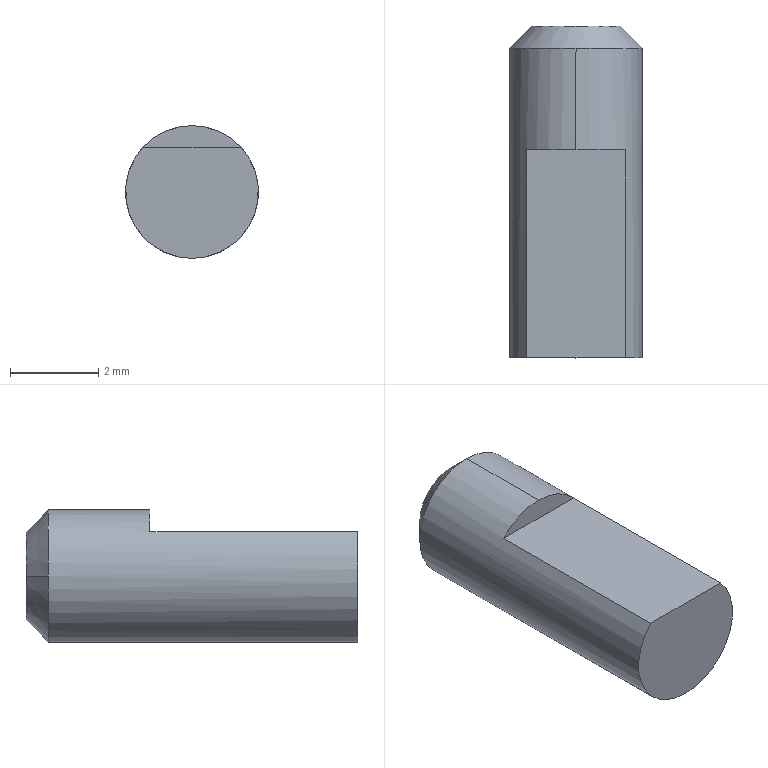Part | NX | 1 solid | 8 faces | box 3 x 7.5 x 3 mm | volume 48.328 mm3 | plane 4 | cylinder 2 | cone 2 | commonest cylinder face diameters 3 x2
STEP:
#1=CARTESIAN_POINT('',(0.171,-56.129,15.403));
#2=VERTEX_POINT('',#1);
#3=CARTESIAN_POINT('',(-1.329,-56.129,16.903));
#4=VERTEX_POINT('',#3);
#5=CARTESIAN_POINT('',(-1.329,-56.129,15.403));
#6=DIRECTION('',(0.,-1.,0.));
#7=DIRECTION('',(1.,0.,0.));
#8=AXIS2_PLACEMENT_3D('',#5,#6,#7);
#9=CIRCLE('',#8,1.5);
#10=EDGE_CURVE('',#2,#4,#9,.T.);
#11=ORIENTED_EDGE('',*,*,#10,.T.);
#12=CARTESIAN_POINT('',(-1.329,-58.429,16.903));
#13=VERTEX_POINT('',#12);
#14=CARTESIAN_POINT('',(-1.329,-63.129,16.903));
#15=DIRECTION('',(0.,-1.,0.));
#16=VECTOR('',#15,1000.);
#17=LINE('',#14,#16);
#18=EDGE_CURVE('',#4,#13,#17,.T.);
#19=ORIENTED_EDGE('',*,*,#18,.T.);
#20=CARTESIAN_POINT('',(-0.211,-58.429,16.403));
#21=VERTEX_POINT('',#20);
#22=CARTESIAN_POINT('',(-1.329,-58.429,15.403));
#23=DIRECTION('',(0.,-1.,0.));
#24=DIRECTION('',(0.,0.,1.));
#25=AXIS2_PLACEMENT_3D('',#22,#23,#24);
#26=CIRCLE('',#25,1.5);
#27=EDGE_CURVE('',#21,#13,#26,.T.);
#28=ORIENTED_EDGE('',*,*,#27,.F.);
#29=CARTESIAN_POINT('',(-0.211,-63.129,16.403));
#30=VERTEX_POINT('',#29);
#31=CARTESIAN_POINT('',(-0.211,-63.129,16.403));
#32=DIRECTION('',(0.,-1.,0.));
#33=VECTOR('',#32,1000.);
#34=LINE('',#31,#33);
#35=EDGE_CURVE('',#21,#30,#34,.T.);
#36=ORIENTED_EDGE('',*,*,#35,.T.);
#37=CARTESIAN_POINT('',(-1.329,-63.129,13.903));
#38=VERTEX_POINT('',#37);
#39=CARTESIAN_POINT('',(-1.329,-63.129,15.403));
#40=DIRECTION('',(0.,-1.,0.));
#41=DIRECTION('',(0.,0.,1.));
#42=AXIS2_PLACEMENT_3D('',#39,#40,#41);
#43=CIRCLE('',#42,1.5);
#44=EDGE_CURVE('',#38,#30,#43,.T.);
#45=ORIENTED_EDGE('',*,*,#44,.F.);
#46=CARTESIAN_POINT('',(-1.329,-56.129,13.903));
#47=VERTEX_POINT('',#46);
#48=CARTESIAN_POINT('',(-1.329,-63.129,13.903));
#49=DIRECTION('',(0.,-1.,0.));
#50=VECTOR('',#49,1000.);
#51=LINE('',#48,#50);
#52=EDGE_CURVE('',#47,#38,#51,.T.);
#53=ORIENTED_EDGE('',*,*,#52,.F.);
#54=CARTESIAN_POINT('',(-1.329,-56.129,15.403));
#55=DIRECTION('',(0.,-1.,0.));
#56=DIRECTION('',(1.,0.,0.));
#57=AXIS2_PLACEMENT_3D('',#54,#55,#56);
#58=CIRCLE('',#57,1.5);
#59=EDGE_CURVE('',#47,#2,#58,.T.);
#60=ORIENTED_EDGE('',*,*,#59,.T.);
#61=EDGE_LOOP('',(#11,#19,#28,#36,#45,#53,#60));
#62=FACE_BOUND('',#61,.T.);
#63=CARTESIAN_POINT('',(-1.329,-63.129,15.403));
#64=DIRECTION('',(0.,-1.,0.));
#65=DIRECTION('',(0.,0.,1.));
#66=AXIS2_PLACEMENT_3D('',#63,#64,#65);
#67=CYLINDRICAL_SURFACE('',#66,1.5);
#68=ADVANCED_FACE('',(#62),#67,.T.);
#69=CARTESIAN_POINT('',(-2.447,-58.429,16.403));
#70=VERTEX_POINT('',#69);
#71=CARTESIAN_POINT('',(-1.329,-58.429,15.403));
#72=DIRECTION('',(0.,-1.,0.));
#73=DIRECTION('',(0.,0.,1.));
#74=AXIS2_PLACEMENT_3D('',#71,#72,#73);
#75=CIRCLE('',#74,1.5);
#76=EDGE_CURVE('',#13,#70,#75,.T.);
#77=ORIENTED_EDGE('',*,*,#76,.F.);
#78=ORIENTED_EDGE('',*,*,#18,.F.);
#79=CARTESIAN_POINT('',(-2.829,-56.129,15.403));
#80=VERTEX_POINT('',#79);
#81=CARTESIAN_POINT('',(-1.329,-56.129,15.403));
#82=DIRECTION('',(0.,-1.,0.));
#83=DIRECTION('',(1.,0.,0.));
#84=AXIS2_PLACEMENT_3D('',#81,#82,#83);
#85=CIRCLE('',#84,1.5);
#86=EDGE_CURVE('',#4,#80,#85,.T.);
#87=ORIENTED_EDGE('',*,*,#86,.T.);
#88=CARTESIAN_POINT('',(-1.329,-56.129,15.403));
#89=DIRECTION('',(0.,-1.,0.));
#90=DIRECTION('',(1.,0.,0.));
#91=AXIS2_PLACEMENT_3D('',#88,#89,#90);
#92=CIRCLE('',#91,1.5);
#93=EDGE_CURVE('',#80,#47,#92,.T.);
#94=ORIENTED_EDGE('',*,*,#93,.T.);
#95=ORIENTED_EDGE('',*,*,#52,.T.);
#96=CARTESIAN_POINT('',(-2.447,-63.129,16.403));
#97=VERTEX_POINT('',#96);
#98=CARTESIAN_POINT('',(-1.329,-63.129,15.403));
#99=DIRECTION('',(0.,-1.,0.));
#100=DIRECTION('',(0.,0.,1.));
#101=AXIS2_PLACEMENT_3D('',#98,#99,#100);
#102=CIRCLE('',#101,1.5);
#103=EDGE_CURVE('',#97,#38,#102,.T.);
#104=ORIENTED_EDGE('',*,*,#103,.F.);
#105=CARTESIAN_POINT('',(-2.447,-63.129,16.403));
#106=DIRECTION('',(0.,-1.,0.));
#107=VECTOR('',#106,1000.);
#108=LINE('',#105,#107);
#109=EDGE_CURVE('',#70,#97,#108,.T.);
#110=ORIENTED_EDGE('',*,*,#109,.F.);
#111=EDGE_LOOP('',(#77,#78,#87,#94,#95,#104,#110));
#112=FACE_BOUND('',#111,.T.);
#113=CARTESIAN_POINT('',(-1.329,-63.129,15.403));
#114=DIRECTION('',(0.,-1.,0.));
#115=DIRECTION('',(0.,0.,1.));
#116=AXIS2_PLACEMENT_3D('',#113,#114,#115);
#117=CYLINDRICAL_SURFACE('',#116,1.5);
#118=ADVANCED_FACE('',(#112),#117,.T.);
#119=CARTESIAN_POINT('',(-0.329,-55.629,15.403));
#120=VERTEX_POINT('',#119);
#121=CARTESIAN_POINT('',(-2.329,-55.629,15.403));
#122=VERTEX_POINT('',#121);
#123=CARTESIAN_POINT('',(-1.329,-55.629,15.403));
#124=DIRECTION('',(0.,-1.,0.));
#125=DIRECTION('',(1.,0.,0.));
#126=AXIS2_PLACEMENT_3D('',#123,#124,#125);
#127=CIRCLE('',#126,1.);
#128=EDGE_CURVE('',#120,#122,#127,.T.);
#129=ORIENTED_EDGE('',*,*,#128,.F.);
#130=CARTESIAN_POINT('',(-1.329,-55.629,15.403));
#131=DIRECTION('',(0.,-1.,0.));
#132=DIRECTION('',(1.,0.,0.));
#133=AXIS2_PLACEMENT_3D('',#130,#131,#132);
#134=CIRCLE('',#133,1.);
#135=EDGE_CURVE('',#122,#120,#134,.T.);
#136=ORIENTED_EDGE('',*,*,#135,.F.);
#137=EDGE_LOOP('',(#129,#136));
#138=FACE_BOUND('',#137,.T.);
#139=CARTESIAN_POINT('',(4.423,-55.629,12.937));
#140=DIRECTION('',(0.,-1.,0.));
#141=DIRECTION('',(-1.,0.,0.));
#142=AXIS2_PLACEMENT_3D('',#139,#140,#141);
#143=PLANE('',#142);
#144=ADVANCED_FACE('',(#138),#143,.F.);
#145=ORIENTED_EDGE('',*,*,#128,.T.);
#146=CARTESIAN_POINT('',(-2.329,-55.629,15.403));
#147=DIRECTION('',(-0.7071,-0.7071,0.));
#148=VECTOR('',#147,1000.);
#149=LINE('',#146,#148);
#150=EDGE_CURVE('',#122,#80,#149,.T.);
#151=ORIENTED_EDGE('',*,*,#150,.T.);
#152=ORIENTED_EDGE('',*,*,#86,.F.);
#153=ORIENTED_EDGE('',*,*,#10,.F.);
#154=CARTESIAN_POINT('',(-0.329,-55.629,15.403));
#155=DIRECTION('',(0.7071,-0.7071,0.));
#156=VECTOR('',#155,1000.);
#157=LINE('',#154,#156);
#158=EDGE_CURVE('',#120,#2,#157,.T.);
#159=ORIENTED_EDGE('',*,*,#158,.F.);
#160=EDGE_LOOP('',(#145,#151,#152,#153,#159));
#161=FACE_BOUND('',#160,.T.);
#162=CARTESIAN_POINT('',(-1.329,-55.629,15.403));
#163=DIRECTION('',(0.,-1.,0.));
#164=DIRECTION('',(1.,0.,0.));
#165=AXIS2_PLACEMENT_3D('',#162,#163,#164);
#166=CONICAL_SURFACE('',#165,1.,0.7854);
#167=ADVANCED_FACE('',(#161),#166,.T.);
#168=ORIENTED_EDGE('',*,*,#158,.T.);
#169=ORIENTED_EDGE('',*,*,#59,.F.);
#170=ORIENTED_EDGE('',*,*,#93,.F.);
#171=ORIENTED_EDGE('',*,*,#150,.F.);
#172=ORIENTED_EDGE('',*,*,#135,.T.);
#173=EDGE_LOOP('',(#168,#169,#170,#171,#172));
#174=FACE_BOUND('',#173,.T.);
#175=CARTESIAN_POINT('',(-1.329,-55.629,15.403));
#176=DIRECTION('',(0.,-1.,0.));
#177=DIRECTION('',(1.,0.,0.));
#178=AXIS2_PLACEMENT_3D('',#175,#176,#177);
#179=CONICAL_SURFACE('',#178,1.,0.7854);
#180=ADVANCED_FACE('',(#174),#179,.T.);
#181=CARTESIAN_POINT('',(4.423,-63.129,16.403));
#182=DIRECTION('',(-1.,0.,0.));
#183=VECTOR('',#182,1000.);
#184=LINE('',#181,#183);
#185=EDGE_CURVE('',#30,#97,#184,.T.);
#186=ORIENTED_EDGE('',*,*,#185,.T.);
#187=ORIENTED_EDGE('',*,*,#103,.T.);
#188=ORIENTED_EDGE('',*,*,#44,.T.);
#189=EDGE_LOOP('',(#186,#187,#188));
#190=FACE_BOUND('',#189,.T.);
#191=CARTESIAN_POINT('',(4.423,-63.129,12.937));
#192=DIRECTION('',(0.,-1.,0.));
#193=DIRECTION('',(-1.,0.,0.));
#194=AXIS2_PLACEMENT_3D('',#191,#192,#193);
#195=PLANE('',#194);
#196=ADVANCED_FACE('',(#190),#195,.T.);
#197=ORIENTED_EDGE('',*,*,#35,.F.);
#198=CARTESIAN_POINT('',(4.423,-58.429,16.403));
#199=DIRECTION('',(-1.,0.,0.));
#200=VECTOR('',#199,1000.);
#201=LINE('',#198,#200);
#202=EDGE_CURVE('',#21,#70,#201,.T.);
#203=ORIENTED_EDGE('',*,*,#202,.T.);
#204=ORIENTED_EDGE('',*,*,#109,.T.);
#205=ORIENTED_EDGE('',*,*,#185,.F.);
#206=EDGE_LOOP('',(#197,#203,#204,#205));
#207=FACE_BOUND('',#206,.T.);
#208=CARTESIAN_POINT('',(-7.654,-60.857,16.403));
#209=DIRECTION('',(0.,0.,1.));
#210=DIRECTION('',(1.,0.,0.));
#211=AXIS2_PLACEMENT_3D('',#208,#209,#210);
#212=PLANE('',#211);
#213=ADVANCED_FACE('',(#207),#212,.T.);
#214=ORIENTED_EDGE('',*,*,#76,.T.);
#215=ORIENTED_EDGE('',*,*,#202,.F.);
#216=ORIENTED_EDGE('',*,*,#27,.T.);
#217=EDGE_LOOP('',(#214,#215,#216));
#218=FACE_BOUND('',#217,.T.);
#219=CARTESIAN_POINT('',(0.171,-58.429,20.403));
#220=DIRECTION('',(0.,1.,0.));
#221=DIRECTION('',(1.,0.,0.));
#222=AXIS2_PLACEMENT_3D('',#219,#220,#221);
#223=PLANE('',#222);
#224=ADVANCED_FACE('',(#218),#223,.F.);
#225=CLOSED_SHELL('',(#68,#118,#144,#167,#180,#196,#213,#224));
#226=MANIFOLD_SOLID_BREP('',#225);
#227=(LENGTH_UNIT()NAMED_UNIT(*)SI_UNIT(.MILLI.,.METRE.));
#228=UNCERTAINTY_MEASURE_WITH_UNIT(LENGTH_MEASURE(0.00001),#227,'','');
#229=(NAMED_UNIT(*)PLANE_ANGLE_UNIT()SI_UNIT($,.RADIAN.));
#230=(NAMED_UNIT(*)SI_UNIT($,.STERADIAN.)SOLID_ANGLE_UNIT());
#231=(GEOMETRIC_REPRESENTATION_CONTEXT(3)GLOBAL_UNCERTAINTY_ASSIGNED_CONTEXT((#228))GLOBAL_UNIT_ASSIGNED_CONTEXT((#227,#229,#230))REPRESENTATION_CONTEXT('',''));
#232=ADVANCED_BREP_SHAPE_REPRESENTATION('',(#226),#231);